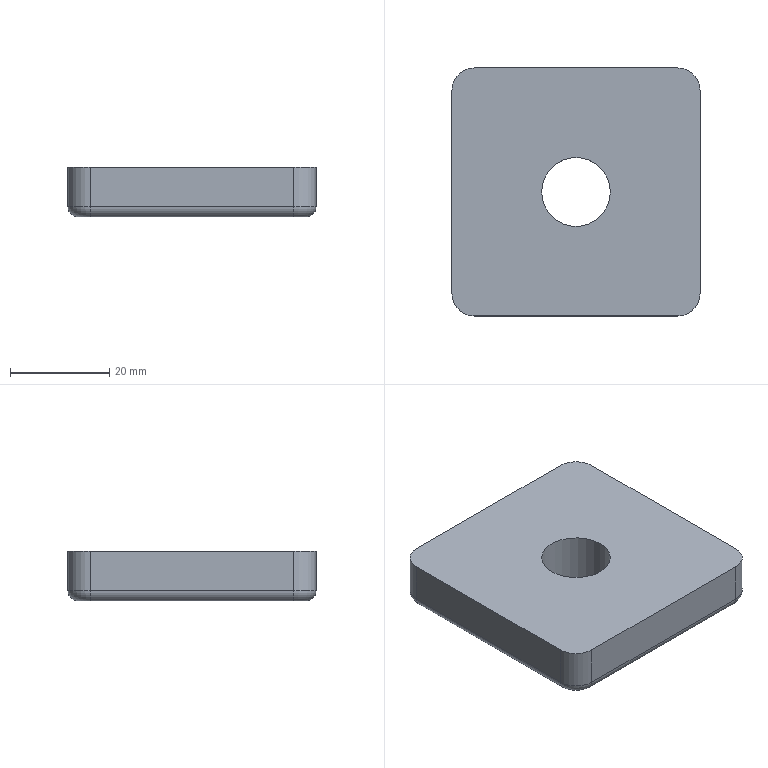Part | STEP file | 14831 | 1 solid | 19 faces | box 50 x 50 x 10 mm | volume 23160 mm3 | cylinder 8 | plane 6 | torus 4 | spline 1 | commonest cylinder face diameters 4 x4 9 x4
STEP:
#1=CARTESIAN_POINT('',(0.,0.,0.));
#2=DIRECTION('',(0.,0.,1.));
#3=DIRECTION('',(1.,0.,0.));
#4=AXIS2_PLACEMENT_3D('',#1,#2,#3);
#5=CARTESIAN_POINT('',(-133.276,-146.636,0.));
#6=VERTEX_POINT('',#5);
#7=CARTESIAN_POINT('',(-133.276,-148.636,2.));
#8=VERTEX_POINT('',#7);
#9=CARTESIAN_POINT('',(-133.276,-146.636,2.));
#10=DIRECTION('',(-1.,0.,0.));
#11=DIRECTION('',(0.,0.,-1.));
#12=AXIS2_PLACEMENT_3D('',#9,#10,#11);
#13=CIRCLE('',#12,2.);
#14=CARTESIAN_POINT('',(-143.526,-146.636,2.));
#15=DIRECTION('',(-1.,0.,0.));
#16=DIRECTION('',(0.,-0.7071,-0.7071));
#17=AXIS2_PLACEMENT_3D('',#14,#15,#16);
#18=CYLINDRICAL_SURFACE('',#17,2.);
#19=CARTESIAN_POINT('',(5.498,-10.25));
#20=DIRECTION('',(1.,0.));
#21=VECTOR('',#20,1.);
#22=LINE('',#19,#21);
#23=(GEOMETRIC_REPRESENTATION_CONTEXT(2)PARAMETRIC_REPRESENTATION_CONTEXT()REPRESENTATION_CONTEXT('',''));
#24=DEFINITIONAL_REPRESENTATION('',(#22),#23);
#25=PCURVE('',#18,#24);
#26=CARTESIAN_POINT('',(-133.276,-144.136,2.));
#27=DIRECTION('',(0.,0.,-1.));
#28=DIRECTION('',(-1.,0.,0.));
#29=AXIS2_PLACEMENT_3D('',#26,#27,#28);
#30=TOROIDAL_SURFACE('',#29,2.5,2.);
#31=CARTESIAN_POINT('',(4.712,1.571));
#32=DIRECTION('',(0.,-1.));
#33=VECTOR('',#32,1.);
#34=LINE('',#31,#33);
#35=(GEOMETRIC_REPRESENTATION_CONTEXT(2)PARAMETRIC_REPRESENTATION_CONTEXT()REPRESENTATION_CONTEXT('',''));
#36=DEFINITIONAL_REPRESENTATION('',(#34),#35);
#37=PCURVE('',#30,#36);
#38=SURFACE_CURVE('',#13,(#25,#37),.PCURVE_S1.);
#39=EDGE_CURVE('',#6,#8,#38,.T.);
#40=ORIENTED_EDGE('',*,*,#39,.T.);
#41=CARTESIAN_POINT('',(-174.276,-148.636,2.));
#42=VERTEX_POINT('',#41);
#43=CARTESIAN_POINT('',(-133.276,-148.636,2.));
#44=DIRECTION('',(-1.,0.,0.));
#45=VECTOR('',#44,1.);
#46=LINE('',#43,#45);
#47=CARTESIAN_POINT('',(7.069,-10.25));
#48=DIRECTION('',(0.,1.));
#49=VECTOR('',#48,1.);
#50=LINE('',#47,#49);
#51=(GEOMETRIC_REPRESENTATION_CONTEXT(2)PARAMETRIC_REPRESENTATION_CONTEXT()REPRESENTATION_CONTEXT('',''));
#52=DEFINITIONAL_REPRESENTATION('',(#50),#51);
#53=PCURVE('',#18,#52);
#54=CARTESIAN_POINT('',(-133.276,-148.636,0.));
#55=DIRECTION('',(0.,-1.,0.));
#56=DIRECTION('',(0.,0.,-1.));
#57=AXIS2_PLACEMENT_3D('',#54,#55,#56);
#58=PLANE('',#57);
#59=CARTESIAN_POINT('',(-2.,0.));
#60=DIRECTION('',(0.,-1.));
#61=VECTOR('',#60,1.);
#62=LINE('',#59,#61);
#63=(GEOMETRIC_REPRESENTATION_CONTEXT(2)PARAMETRIC_REPRESENTATION_CONTEXT()REPRESENTATION_CONTEXT('',''));
#64=DEFINITIONAL_REPRESENTATION('',(#62),#63);
#65=PCURVE('',#58,#64);
#66=SURFACE_CURVE('',#46,(#53,#65),.PCURVE_S1.);
#67=EDGE_CURVE('',#8,#42,#66,.T.);
#68=ORIENTED_EDGE('',*,*,#67,.T.);
#69=CARTESIAN_POINT('',(-174.276,-146.636,0.));
#70=VERTEX_POINT('',#69);
#71=CARTESIAN_POINT('',(-174.276,-146.636,2.));
#72=DIRECTION('',(1.,0.,0.));
#73=DIRECTION('',(0.,-1.,0.));
#74=AXIS2_PLACEMENT_3D('',#71,#72,#73);
#75=CIRCLE('',#74,2.);
#76=CARTESIAN_POINT('',(7.069,30.75));
#77=DIRECTION('',(-1.,0.));
#78=VECTOR('',#77,1.);
#79=LINE('',#76,#78);
#80=(GEOMETRIC_REPRESENTATION_CONTEXT(2)PARAMETRIC_REPRESENTATION_CONTEXT()REPRESENTATION_CONTEXT('',''));
#81=DEFINITIONAL_REPRESENTATION('',(#79),#80);
#82=PCURVE('',#18,#81);
#83=CARTESIAN_POINT('',(-174.276,-144.136,2.));
#84=DIRECTION('',(0.,0.,-1.));
#85=DIRECTION('',(-1.,0.,0.));
#86=AXIS2_PLACEMENT_3D('',#83,#84,#85);
#87=TOROIDAL_SURFACE('',#86,2.5,2.);
#88=CARTESIAN_POINT('',(4.712,0.));
#89=DIRECTION('',(0.,1.));
#90=VECTOR('',#89,1.);
#91=LINE('',#88,#90);
#92=(GEOMETRIC_REPRESENTATION_CONTEXT(2)PARAMETRIC_REPRESENTATION_CONTEXT()REPRESENTATION_CONTEXT('',''));
#93=DEFINITIONAL_REPRESENTATION('',(#91),#92);
#94=PCURVE('',#87,#93);
#95=SURFACE_CURVE('',#75,(#82,#94),.PCURVE_S1.);
#96=EDGE_CURVE('',#42,#70,#95,.T.);
#97=ORIENTED_EDGE('',*,*,#96,.T.);
#98=CARTESIAN_POINT('',(-174.276,-146.636,0.));
#99=DIRECTION('',(1.,0.,0.));
#100=VECTOR('',#99,1.);
#101=LINE('',#98,#100);
#102=CARTESIAN_POINT('',(5.498,30.75));
#103=DIRECTION('',(0.,-1.));
#104=VECTOR('',#103,1.);
#105=LINE('',#102,#104);
#106=(GEOMETRIC_REPRESENTATION_CONTEXT(2)PARAMETRIC_REPRESENTATION_CONTEXT()REPRESENTATION_CONTEXT('',''));
#107=DEFINITIONAL_REPRESENTATION('',(#105),#106);
#108=PCURVE('',#18,#107);
#109=CARTESIAN_POINT('',(-153.776,-123.636,0.));
#110=DIRECTION('',(0.,0.,1.));
#111=DIRECTION('',(1.,0.,0.));
#112=AXIS2_PLACEMENT_3D('',#109,#110,#111);
#113=PLANE('',#112);
#114=CARTESIAN_POINT('',(-20.5,-23.));
#115=DIRECTION('',(1.,0.));
#116=VECTOR('',#115,1.);
#117=LINE('',#114,#116);
#118=(GEOMETRIC_REPRESENTATION_CONTEXT(2)PARAMETRIC_REPRESENTATION_CONTEXT()REPRESENTATION_CONTEXT('',''));
#119=DEFINITIONAL_REPRESENTATION('',(#117),#118);
#120=PCURVE('',#113,#119);
#121=SURFACE_CURVE('',#101,(#108,#120),.PCURVE_S1.);
#122=EDGE_CURVE('',#70,#6,#121,.T.);
#123=ORIENTED_EDGE('',*,*,#122,.T.);
#124=EDGE_LOOP('',(#40,#68,#97,#123));
#125=FACE_BOUND('',#124,.T.);
#126=ADVANCED_FACE('',(#125),#18,.T.);
#127=CARTESIAN_POINT('',(-130.776,-144.136,0.));
#128=VERTEX_POINT('',#127);
#129=CARTESIAN_POINT('',(-128.776,-144.136,2.));
#130=VERTEX_POINT('',#129);
#131=CARTESIAN_POINT('',(-130.776,-144.136,2.));
#132=DIRECTION('',(0.,-1.,0.));
#133=DIRECTION('',(0.,0.,-1.));
#134=AXIS2_PLACEMENT_3D('',#131,#132,#133);
#135=CIRCLE('',#134,2.);
#136=CARTESIAN_POINT('',(3.142,1.571));
#137=DIRECTION('',(0.,-1.));
#138=VECTOR('',#137,1.);
#139=LINE('',#136,#138);
#140=(GEOMETRIC_REPRESENTATION_CONTEXT(2)PARAMETRIC_REPRESENTATION_CONTEXT()REPRESENTATION_CONTEXT('',''));
#141=DEFINITIONAL_REPRESENTATION('',(#139),#140);
#142=PCURVE('',#30,#141);
#143=CARTESIAN_POINT('',(-130.776,-113.386,2.));
#144=DIRECTION('',(0.,-1.,0.));
#145=DIRECTION('',(0.7071,0.,-0.7071));
#146=AXIS2_PLACEMENT_3D('',#143,#144,#145);
#147=CYLINDRICAL_SURFACE('',#146,2.);
#148=CARTESIAN_POINT('',(5.498,30.75));
#149=DIRECTION('',(1.,0.));
#150=VECTOR('',#149,1.);
#151=LINE('',#148,#150);
#152=(GEOMETRIC_REPRESENTATION_CONTEXT(2)PARAMETRIC_REPRESENTATION_CONTEXT()REPRESENTATION_CONTEXT('',''));
#153=DEFINITIONAL_REPRESENTATION('',(#151),#152);
#154=PCURVE('',#147,#153);
#155=SURFACE_CURVE('',#135,(#142,#154),.PCURVE_S1.);
#156=EDGE_CURVE('',#128,#130,#155,.T.);
#157=ORIENTED_EDGE('',*,*,#156,.T.);
#158=CARTESIAN_POINT('',(-133.276,-144.136,2.));
#159=DIRECTION('',(0.,0.,-1.));
#160=DIRECTION('',(0.7071,-0.7071,0.));
#161=AXIS2_PLACEMENT_3D('',#158,#159,#160);
#162=CIRCLE('',#161,4.5);
#163=CARTESIAN_POINT('',(-2.356,0.));
#164=DIRECTION('',(1.,0.));
#165=VECTOR('',#164,1.);
#166=LINE('',#163,#165);
#167=(GEOMETRIC_REPRESENTATION_CONTEXT(2)PARAMETRIC_REPRESENTATION_CONTEXT()REPRESENTATION_CONTEXT('',''));
#168=DEFINITIONAL_REPRESENTATION('',(#166),#167);
#169=PCURVE('',#30,#168);
#170=CARTESIAN_POINT('',(-133.276,-144.136,0.));
#171=DIRECTION('',(0.,0.,1.));
#172=DIRECTION('',(0.,1.,0.));
#173=AXIS2_PLACEMENT_3D('',#170,#171,#172);
#174=CYLINDRICAL_SURFACE('',#173,4.5);
#175=CARTESIAN_POINT('',(10.21,2.));
#176=DIRECTION('',(-1.,0.));
#177=VECTOR('',#176,1.);
#178=LINE('',#175,#177);
#179=(GEOMETRIC_REPRESENTATION_CONTEXT(2)PARAMETRIC_REPRESENTATION_CONTEXT()REPRESENTATION_CONTEXT('',''));
#180=DEFINITIONAL_REPRESENTATION('',(#178),#179);
#181=PCURVE('',#174,#180);
#182=SURFACE_CURVE('',#162,(#169,#181),.PCURVE_S1.);
#183=EDGE_CURVE('',#130,#8,#182,.T.);
#184=ORIENTED_EDGE('',*,*,#183,.T.);
#185=ORIENTED_EDGE('',*,*,#39,.F.);
#186=CARTESIAN_POINT('',(-133.276,-144.136,0.));
#187=DIRECTION('',(0.,0.,1.));
#188=DIRECTION('',(0.7071,-0.7071,0.));
#189=AXIS2_PLACEMENT_3D('',#186,#187,#188);
#190=CIRCLE('',#189,2.5);
#191=CARTESIAN_POINT('',(10.21,1.571));
#192=DIRECTION('',(-1.,0.));
#193=VECTOR('',#192,1.);
#194=LINE('',#191,#193);
#195=(GEOMETRIC_REPRESENTATION_CONTEXT(2)PARAMETRIC_REPRESENTATION_CONTEXT()REPRESENTATION_CONTEXT('',''));
#196=DEFINITIONAL_REPRESENTATION('',(#194),#195);
#197=PCURVE('',#30,#196);
#198=CARTESIAN_POINT('',(20.5,-20.5));
#199=DIRECTION('',(0.7071,-0.7071));
#200=AXIS2_PLACEMENT_2D('',#198,#199);
#201=CIRCLE('',#200,2.5);
#202=(GEOMETRIC_REPRESENTATION_CONTEXT(2)PARAMETRIC_REPRESENTATION_CONTEXT()REPRESENTATION_CONTEXT('',''));
#203=DEFINITIONAL_REPRESENTATION('',(#201),#202);
#204=PCURVE('',#113,#203);
#205=SURFACE_CURVE('',#190,(#197,#204),.PCURVE_S1.);
#206=EDGE_CURVE('',#6,#128,#205,.T.);
#207=ORIENTED_EDGE('',*,*,#206,.T.);
#208=EDGE_LOOP('',(#157,#184,#185,#207));
#209=FACE_BOUND('',#208,.T.);
#210=ADVANCED_FACE('',(#209),#30,.T.);
#211=CARTESIAN_POINT('',(-178.776,-144.136,2.));
#212=VERTEX_POINT('',#211);
#213=CARTESIAN_POINT('',(-176.776,-144.136,0.));
#214=VERTEX_POINT('',#213);
#215=CARTESIAN_POINT('',(-176.776,-144.136,2.));
#216=DIRECTION('',(0.,-1.,0.));
#217=DIRECTION('',(-1.,0.,0.));
#218=AXIS2_PLACEMENT_3D('',#215,#216,#217);
#219=CIRCLE('',#218,2.);
#220=CARTESIAN_POINT('',(6.283,0.));
#221=DIRECTION('',(0.,1.));
#222=VECTOR('',#221,1.);
#223=LINE('',#220,#222);
#224=(GEOMETRIC_REPRESENTATION_CONTEXT(2)PARAMETRIC_REPRESENTATION_CONTEXT()REPRESENTATION_CONTEXT('',''));
#225=DEFINITIONAL_REPRESENTATION('',(#223),#224);
#226=PCURVE('',#87,#225);
#227=CARTESIAN_POINT('',(-176.776,-133.886,2.));
#228=DIRECTION('',(0.,1.,0.));
#229=DIRECTION('',(-0.7071,0.,-0.7071));
#230=AXIS2_PLACEMENT_3D('',#227,#228,#229);
#231=CYLINDRICAL_SURFACE('',#230,2.);
#232=CARTESIAN_POINT('',(7.069,-10.25));
#233=DIRECTION('',(-1.,0.));
#234=VECTOR('',#233,1.);
#235=LINE('',#232,#234);
#236=(GEOMETRIC_REPRESENTATION_CONTEXT(2)PARAMETRIC_REPRESENTATION_CONTEXT()REPRESENTATION_CONTEXT('',''));
#237=DEFINITIONAL_REPRESENTATION('',(#235),#236);
#238=PCURVE('',#231,#237);
#239=SURFACE_CURVE('',#219,(#226,#238),.PCURVE_S1.);
#240=EDGE_CURVE('',#212,#214,#239,.T.);
#241=ORIENTED_EDGE('',*,*,#240,.T.);
#242=CARTESIAN_POINT('',(-174.276,-144.136,0.));
#243=DIRECTION('',(0.,0.,1.));
#244=DIRECTION('',(-0.7071,-0.7071,0.));
#245=AXIS2_PLACEMENT_3D('',#242,#243,#244);
#246=CIRCLE('',#245,2.5);
#247=CARTESIAN_POINT('',(11.781,1.571));
#248=DIRECTION('',(-1.,0.));
#249=VECTOR('',#248,1.);
#250=LINE('',#247,#249);
#251=(GEOMETRIC_REPRESENTATION_CONTEXT(2)PARAMETRIC_REPRESENTATION_CONTEXT()REPRESENTATION_CONTEXT('',''));
#252=DEFINITIONAL_REPRESENTATION('',(#250),#251);
#253=PCURVE('',#87,#252);
#254=CARTESIAN_POINT('',(-20.5,-20.5));
#255=DIRECTION('',(-0.7071,-0.7071));
#256=AXIS2_PLACEMENT_2D('',#254,#255);
#257=CIRCLE('',#256,2.5);
#258=(GEOMETRIC_REPRESENTATION_CONTEXT(2)PARAMETRIC_REPRESENTATION_CONTEXT()REPRESENTATION_CONTEXT('',''));
#259=DEFINITIONAL_REPRESENTATION('',(#257),#258);
#260=PCURVE('',#113,#259);
#261=SURFACE_CURVE('',#246,(#253,#260),.PCURVE_S1.);
#262=EDGE_CURVE('',#214,#70,#261,.T.);
#263=ORIENTED_EDGE('',*,*,#262,.T.);
#264=ORIENTED_EDGE('',*,*,#96,.F.);
#265=CARTESIAN_POINT('',(-174.276,-144.136,2.));
#266=DIRECTION('',(0.,0.,-1.));
#267=DIRECTION('',(-0.7071,-0.7071,0.));
#268=AXIS2_PLACEMENT_3D('',#265,#266,#267);
#269=CIRCLE('',#268,4.5);
#270=CARTESIAN_POINT('',(-0.7854,0.));
#271=DIRECTION('',(1.,0.));
#272=VECTOR('',#271,1.);
#273=LINE('',#270,#272);
#274=(GEOMETRIC_REPRESENTATION_CONTEXT(2)PARAMETRIC_REPRESENTATION_CONTEXT()REPRESENTATION_CONTEXT('',''));
#275=DEFINITIONAL_REPRESENTATION('',(#273),#274);
#276=PCURVE('',#87,#275);
#277=CARTESIAN_POINT('',(-174.276,-144.136,0.));
#278=DIRECTION('',(0.,0.,1.));
#279=DIRECTION('',(1.,0.,0.));
#280=AXIS2_PLACEMENT_3D('',#277,#278,#279);
#281=CYLINDRICAL_SURFACE('',#280,4.5);
#282=CARTESIAN_POINT('',(10.21,2.));
#283=DIRECTION('',(-1.,0.));
#284=VECTOR('',#283,1.);
#285=LINE('',#282,#284);
#286=(GEOMETRIC_REPRESENTATION_CONTEXT(2)PARAMETRIC_REPRESENTATION_CONTEXT()REPRESENTATION_CONTEXT('',''));
#287=DEFINITIONAL_REPRESENTATION('',(#285),#286);
#288=PCURVE('',#281,#287);
#289=SURFACE_CURVE('',#269,(#276,#288),.PCURVE_S1.);
#290=EDGE_CURVE('',#42,#212,#289,.T.);
#291=ORIENTED_EDGE('',*,*,#290,.T.);
#292=EDGE_LOOP('',(#241,#263,#264,#291));
#293=FACE_BOUND('',#292,.T.);
#294=ADVANCED_FACE('',(#293),#87,.T.);
#295=CARTESIAN_POINT('',(-130.776,-103.136,0.));
#296=VERTEX_POINT('',#295);
#297=CARTESIAN_POINT('',(-128.776,-103.136,2.));
#298=VERTEX_POINT('',#297);
#299=CARTESIAN_POINT('',(-130.776,-103.136,2.));
#300=DIRECTION('',(0.,-1.,0.));
#301=DIRECTION('',(0.,0.,-1.));
#302=AXIS2_PLACEMENT_3D('',#299,#300,#301);
#303=CIRCLE('',#302,2.);
#304=CARTESIAN_POINT('',(5.498,-10.25));
#305=DIRECTION('',(1.,0.));
#306=VECTOR('',#305,1.);
#307=LINE('',#304,#306);
#308=(GEOMETRIC_REPRESENTATION_CONTEXT(2)PARAMETRIC_REPRESENTATION_CONTEXT()REPRESENTATION_CONTEXT('',''));
#309=DEFINITIONAL_REPRESENTATION('',(#307),#308);
#310=PCURVE('',#147,#309);
#311=CARTESIAN_POINT('',(-133.276,-103.136,2.));
#312=DIRECTION('',(0.,0.,-1.));
#313=DIRECTION('',(-1.,0.,0.));
#314=AXIS2_PLACEMENT_3D('',#311,#312,#313);
#315=TOROIDAL_SURFACE('',#314,2.5,2.);
#316=CARTESIAN_POINT('',(3.142,1.571));
#317=DIRECTION('',(0.,-1.));
#318=VECTOR('',#317,1.);
#319=LINE('',#316,#318);
#320=(GEOMETRIC_REPRESENTATION_CONTEXT(2)PARAMETRIC_REPRESENTATION_CONTEXT()REPRESENTATION_CONTEXT('',''));
#321=DEFINITIONAL_REPRESENTATION('',(#319),#320);
#322=PCURVE('',#315,#321);
#323=SURFACE_CURVE('',#303,(#310,#322),.PCURVE_S1.);
#324=EDGE_CURVE('',#296,#298,#323,.T.);
#325=ORIENTED_EDGE('',*,*,#324,.T.);
#326=CARTESIAN_POINT('',(-128.776,-103.136,2.));
#327=DIRECTION('',(0.,-1.,0.));
#328=VECTOR('',#327,1.);
#329=LINE('',#326,#328);
#330=CARTESIAN_POINT('',(7.069,-10.25));
#331=DIRECTION('',(0.,1.));
#332=VECTOR('',#331,1.);
#333=LINE('',#330,#332);
#334=(GEOMETRIC_REPRESENTATION_CONTEXT(2)PARAMETRIC_REPRESENTATION_CONTEXT()REPRESENTATION_CONTEXT('',''));
#335=DEFINITIONAL_REPRESENTATION('',(#333),#334);
#336=PCURVE('',#147,#335);
#337=CARTESIAN_POINT('',(-128.776,-103.136,0.));
#338=DIRECTION('',(1.,0.,0.));
#339=DIRECTION('',(0.,0.,-1.));
#340=AXIS2_PLACEMENT_3D('',#337,#338,#339);
#341=PLANE('',#340);
#342=CARTESIAN_POINT('',(-2.,0.));
#343=DIRECTION('',(0.,-1.));
#344=VECTOR('',#343,1.);
#345=LINE('',#342,#344);
#346=(GEOMETRIC_REPRESENTATION_CONTEXT(2)PARAMETRIC_REPRESENTATION_CONTEXT()REPRESENTATION_CONTEXT('',''));
#347=DEFINITIONAL_REPRESENTATION('',(#345),#346);
#348=PCURVE('',#341,#347);
#349=SURFACE_CURVE('',#329,(#336,#348),.PCURVE_S1.);
#350=EDGE_CURVE('',#298,#130,#349,.T.);
#351=ORIENTED_EDGE('',*,*,#350,.T.);
#352=ORIENTED_EDGE('',*,*,#156,.F.);
#353=CARTESIAN_POINT('',(-130.776,-144.136,0.));
#354=DIRECTION('',(0.,1.,0.));
#355=VECTOR('',#354,1.);
#356=LINE('',#353,#355);
#357=CARTESIAN_POINT('',(5.498,30.75));
#358=DIRECTION('',(0.,-1.));
#359=VECTOR('',#358,1.);
#360=LINE('',#357,#359);
#361=(GEOMETRIC_REPRESENTATION_CONTEXT(2)PARAMETRIC_REPRESENTATION_CONTEXT()REPRESENTATION_CONTEXT('',''));
#362=DEFINITIONAL_REPRESENTATION('',(#360),#361);
#363=PCURVE('',#147,#362);
#364=CARTESIAN_POINT('',(23.,-20.5));
#365=DIRECTION('',(0.,1.));
#366=VECTOR('',#365,1.);
#367=LINE('',#364,#366);
#368=(GEOMETRIC_REPRESENTATION_CONTEXT(2)PARAMETRIC_REPRESENTATION_CONTEXT()REPRESENTATION_CONTEXT('',''));
#369=DEFINITIONAL_REPRESENTATION('',(#367),#368);
#370=PCURVE('',#113,#369);
#371=SURFACE_CURVE('',#356,(#363,#370),.PCURVE_S1.);
#372=EDGE_CURVE('',#128,#296,#371,.T.);
#373=ORIENTED_EDGE('',*,*,#372,.T.);
#374=EDGE_LOOP('',(#325,#351,#352,#373));
#375=FACE_BOUND('',#374,.T.);
#376=ADVANCED_FACE('',(#375),#147,.T.);
#377=CARTESIAN_POINT('',(-178.776,-103.136,2.));
#378=VERTEX_POINT('',#377);
#379=CARTESIAN_POINT('',(-176.776,-103.136,0.));
#380=VERTEX_POINT('',#379);
#381=CARTESIAN_POINT('',(-176.776,-103.136,2.));
#382=DIRECTION('',(0.,-1.,0.));
#383=DIRECTION('',(-1.,0.,0.));
#384=AXIS2_PLACEMENT_3D('',#381,#382,#383);
#385=CIRCLE('',#384,2.);
#386=CARTESIAN_POINT('',(7.069,30.75));
#387=DIRECTION('',(-1.,0.));
#388=VECTOR('',#387,1.);
#389=LINE('',#386,#388);
#390=(GEOMETRIC_REPRESENTATION_CONTEXT(2)PARAMETRIC_REPRESENTATION_CONTEXT()REPRESENTATION_CONTEXT('',''));
#391=DEFINITIONAL_REPRESENTATION('',(#389),#390);
#392=PCURVE('',#231,#391);
#393=CARTESIAN_POINT('',(-174.276,-103.136,2.));
#394=DIRECTION('',(0.,0.,-1.));
#395=DIRECTION('',(-1.,0.,0.));
#396=AXIS2_PLACEMENT_3D('',#393,#394,#395);
#397=TOROIDAL_SURFACE('',#396,2.5,2.);
#398=CARTESIAN_POINT('',(0.,0.));
#399=DIRECTION('',(0.,1.));
#400=VECTOR('',#399,1.);
#401=LINE('',#398,#400);
#402=(GEOMETRIC_REPRESENTATION_CONTEXT(2)PARAMETRIC_REPRESENTATION_CONTEXT()REPRESENTATION_CONTEXT('',''));
#403=DEFINITIONAL_REPRESENTATION('',(#401),#402);
#404=PCURVE('',#397,#403);
#405=SURFACE_CURVE('',#385,(#392,#404),.PCURVE_S1.);
#406=EDGE_CURVE('',#378,#380,#405,.T.);
#407=ORIENTED_EDGE('',*,*,#406,.T.);
#408=CARTESIAN_POINT('',(-176.776,-103.136,0.));
#409=DIRECTION('',(0.,-1.,0.));
#410=VECTOR('',#409,1.);
#411=LINE('',#408,#410);
#412=CARTESIAN_POINT('',(5.498,30.75));
#413=DIRECTION('',(0.,-1.));
#414=VECTOR('',#413,1.);
#415=LINE('',#412,#414);
#416=(GEOMETRIC_REPRESENTATION_CONTEXT(2)PARAMETRIC_REPRESENTATION_CONTEXT()REPRESENTATION_CONTEXT('',''));
#417=DEFINITIONAL_REPRESENTATION('',(#415),#416);
#418=PCURVE('',#231,#417);
#419=CARTESIAN_POINT('',(-23.,20.5));
#420=DIRECTION('',(0.,-1.));
#421=VECTOR('',#420,1.);
#422=LINE('',#419,#421);
#423=(GEOMETRIC_REPRESENTATION_CONTEXT(2)PARAMETRIC_REPRESENTATION_CONTEXT()REPRESENTATION_CONTEXT('',''));
#424=DEFINITIONAL_REPRESENTATION('',(#422),#423);
#425=PCURVE('',#113,#424);
#426=SURFACE_CURVE('',#411,(#418,#425),.PCURVE_S1.);
#427=EDGE_CURVE('',#380,#214,#426,.T.);
#428=ORIENTED_EDGE('',*,*,#427,.T.);
#429=ORIENTED_EDGE('',*,*,#240,.F.);
#430=CARTESIAN_POINT('',(-178.776,-144.136,2.));
#431=DIRECTION('',(0.,1.,0.));
#432=VECTOR('',#431,1.);
#433=LINE('',#430,#432);
#434=CARTESIAN_POINT('',(7.069,-10.25));
#435=DIRECTION('',(0.,1.));
#436=VECTOR('',#435,1.);
#437=LINE('',#434,#436);
#438=(GEOMETRIC_REPRESENTATION_CONTEXT(2)PARAMETRIC_REPRESENTATION_CONTEXT()REPRESENTATION_CONTEXT('',''));
#439=DEFINITIONAL_REPRESENTATION('',(#437),#438);
#440=PCURVE('',#231,#439);
#441=CARTESIAN_POINT('',(-178.776,-144.136,0.));
#442=DIRECTION('',(-1.,0.,0.));
#443=DIRECTION('',(0.,0.,1.));
#444=AXIS2_PLACEMENT_3D('',#441,#442,#443);
#445=PLANE('',#444);
#446=CARTESIAN_POINT('',(2.,0.));
#447=DIRECTION('',(0.,1.));
#448=VECTOR('',#447,1.);
#449=LINE('',#446,#448);
#450=(GEOMETRIC_REPRESENTATION_CONTEXT(2)PARAMETRIC_REPRESENTATION_CONTEXT()REPRESENTATION_CONTEXT('',''));
#451=DEFINITIONAL_REPRESENTATION('',(#449),#450);
#452=PCURVE('',#445,#451);
#453=SURFACE_CURVE('',#433,(#440,#452),.PCURVE_S1.);
#454=EDGE_CURVE('',#212,#378,#453,.T.);
#455=ORIENTED_EDGE('',*,*,#454,.T.);
#456=EDGE_LOOP('',(#407,#428,#429,#455));
#457=FACE_BOUND('',#456,.T.);
#458=ADVANCED_FACE('',(#457),#231,.T.);
#459=CARTESIAN_POINT('',(-133.276,-100.636,0.));
#460=VERTEX_POINT('',#459);
#461=CARTESIAN_POINT('',(-133.276,-98.636,2.));
#462=VERTEX_POINT('',#461);
#463=CARTESIAN_POINT('',(-133.276,-100.636,2.));
#464=DIRECTION('',(1.,0.,0.));
#465=DIRECTION('',(0.,0.,-1.));
#466=AXIS2_PLACEMENT_3D('',#463,#464,#465);
#467=CIRCLE('',#466,2.);
#468=CARTESIAN_POINT('',(1.571,1.571));
#469=DIRECTION('',(0.,-1.));
#470=VECTOR('',#469,1.);
#471=LINE('',#468,#470);
#472=(GEOMETRIC_REPRESENTATION_CONTEXT(2)PARAMETRIC_REPRESENTATION_CONTEXT()REPRESENTATION_CONTEXT('',''));
#473=DEFINITIONAL_REPRESENTATION('',(#471),#472);
#474=PCURVE('',#315,#473);
#475=CARTESIAN_POINT('',(-164.026,-100.636,2.));
#476=DIRECTION('',(1.,0.,0.));
#477=DIRECTION('',(0.,0.7071,-0.7071));
#478=AXIS2_PLACEMENT_3D('',#475,#476,#477);
#479=CYLINDRICAL_SURFACE('',#478,2.);
#480=CARTESIAN_POINT('',(5.498,30.75));
#481=DIRECTION('',(1.,0.));
#482=VECTOR('',#481,1.);
#483=LINE('',#480,#482);
#484=(GEOMETRIC_REPRESENTATION_CONTEXT(2)PARAMETRIC_REPRESENTATION_CONTEXT()REPRESENTATION_CONTEXT('',''));
#485=DEFINITIONAL_REPRESENTATION('',(#483),#484);
#486=PCURVE('',#479,#485);
#487=SURFACE_CURVE('',#467,(#474,#486),.PCURVE_S1.);
#488=EDGE_CURVE('',#460,#462,#487,.T.);
#489=ORIENTED_EDGE('',*,*,#488,.T.);
#490=CARTESIAN_POINT('',(-133.276,-103.136,2.));
#491=DIRECTION('',(0.,0.,-1.));
#492=DIRECTION('',(0.7071,0.7071,0.));
#493=AXIS2_PLACEMENT_3D('',#490,#491,#492);
#494=CIRCLE('',#493,4.5);
#495=CARTESIAN_POINT('',(-3.927,0.));
#496=DIRECTION('',(1.,0.));
#497=VECTOR('',#496,1.);
#498=LINE('',#495,#497);
#499=(GEOMETRIC_REPRESENTATION_CONTEXT(2)PARAMETRIC_REPRESENTATION_CONTEXT()REPRESENTATION_CONTEXT('',''));
#500=DEFINITIONAL_REPRESENTATION('',(#498),#499);
#501=PCURVE('',#315,#500);
#502=CARTESIAN_POINT('',(-133.276,-103.136,0.));
#503=DIRECTION('',(0.,0.,1.));
#504=DIRECTION('',(-1.,0.,0.));
#505=AXIS2_PLACEMENT_3D('',#502,#503,#504);
#506=CYLINDRICAL_SURFACE('',#505,4.5);
#507=CARTESIAN_POINT('',(10.21,2.));
#508=DIRECTION('',(-1.,0.));
#509=VECTOR('',#508,1.);
#510=LINE('',#507,#509);
#511=(GEOMETRIC_REPRESENTATION_CONTEXT(2)PARAMETRIC_REPRESENTATION_CONTEXT()REPRESENTATION_CONTEXT('',''));
#512=DEFINITIONAL_REPRESENTATION('',(#510),#511);
#513=PCURVE('',#506,#512);
#514=SURFACE_CURVE('',#494,(#501,#513),.PCURVE_S1.);
#515=EDGE_CURVE('',#462,#298,#514,.T.);
#516=ORIENTED_EDGE('',*,*,#515,.T.);
#517=ORIENTED_EDGE('',*,*,#324,.F.);
#518=CARTESIAN_POINT('',(-133.276,-103.136,0.));
#519=DIRECTION('',(0.,0.,1.));
#520=DIRECTION('',(0.7071,0.7071,0.));
#521=AXIS2_PLACEMENT_3D('',#518,#519,#520);
#522=CIRCLE('',#521,2.5);
#523=CARTESIAN_POINT('',(8.639,1.571));
#524=DIRECTION('',(-1.,0.));
#525=VECTOR('',#524,1.);
#526=LINE('',#523,#525);
#527=(GEOMETRIC_REPRESENTATION_CONTEXT(2)PARAMETRIC_REPRESENTATION_CONTEXT()REPRESENTATION_CONTEXT('',''));
#528=DEFINITIONAL_REPRESENTATION('',(#526),#527);
#529=PCURVE('',#315,#528);
#530=CARTESIAN_POINT('',(20.5,20.5));
#531=DIRECTION('',(0.7071,0.7071));
#532=AXIS2_PLACEMENT_2D('',#530,#531);
#533=CIRCLE('',#532,2.5);
#534=(GEOMETRIC_REPRESENTATION_CONTEXT(2)PARAMETRIC_REPRESENTATION_CONTEXT()REPRESENTATION_CONTEXT('',''));
#535=DEFINITIONAL_REPRESENTATION('',(#533),#534);
#536=PCURVE('',#113,#535);
#537=SURFACE_CURVE('',#522,(#529,#536),.PCURVE_S1.);
#538=EDGE_CURVE('',#296,#460,#537,.T.);
#539=ORIENTED_EDGE('',*,*,#538,.T.);
#540=EDGE_LOOP('',(#489,#516,#517,#539));
#541=FACE_BOUND('',#540,.T.);
#542=ADVANCED_FACE('',(#541),#315,.T.);
#543=CARTESIAN_POINT('',(-174.276,-98.636,2.));
#544=VERTEX_POINT('',#543);
#545=CARTESIAN_POINT('',(-174.276,-100.636,0.));
#546=VERTEX_POINT('',#545);
#547=CARTESIAN_POINT('',(-174.276,-100.636,2.));
#548=DIRECTION('',(-1.,0.,0.));
#549=DIRECTION('',(0.,1.,0.));
#550=AXIS2_PLACEMENT_3D('',#547,#548,#549);
#551=CIRCLE('',#550,2.);
#552=CARTESIAN_POINT('',(1.571,0.));
#553=DIRECTION('',(0.,1.));
#554=VECTOR('',#553,1.);
#555=LINE('',#552,#554);
#556=(GEOMETRIC_REPRESENTATION_CONTEXT(2)PARAMETRIC_REPRESENTATION_CONTEXT()REPRESENTATION_CONTEXT('',''));
#557=DEFINITIONAL_REPRESENTATION('',(#555),#556);
#558=PCURVE('',#397,#557);
#559=CARTESIAN_POINT('',(7.069,-10.25));
#560=DIRECTION('',(-1.,0.));
#561=VECTOR('',#560,1.);
#562=LINE('',#559,#561);
#563=(GEOMETRIC_REPRESENTATION_CONTEXT(2)PARAMETRIC_REPRESENTATION_CONTEXT()REPRESENTATION_CONTEXT('',''));
#564=DEFINITIONAL_REPRESENTATION('',(#562),#563);
#565=PCURVE('',#479,#564);
#566=SURFACE_CURVE('',#551,(#558,#565),.PCURVE_S1.);
#567=EDGE_CURVE('',#544,#546,#566,.T.);
#568=ORIENTED_EDGE('',*,*,#567,.T.);
#569=CARTESIAN_POINT('',(-174.276,-103.136,0.));
#570=DIRECTION('',(0.,0.,1.));
#571=DIRECTION('',(-0.7071,0.7071,0.));
#572=AXIS2_PLACEMENT_3D('',#569,#570,#571);
#573=CIRCLE('',#572,2.5);
#574=CARTESIAN_POINT('',(7.069,1.571));
#575=DIRECTION('',(-1.,0.));
#576=VECTOR('',#575,1.);
#577=LINE('',#574,#576);
#578=(GEOMETRIC_REPRESENTATION_CONTEXT(2)PARAMETRIC_REPRESENTATION_CONTEXT()REPRESENTATION_CONTEXT('',''));
#579=DEFINITIONAL_REPRESENTATION('',(#577),#578);
#580=PCURVE('',#397,#579);
#581=CARTESIAN_POINT('',(-20.5,20.5));
#582=DIRECTION('',(-0.7071,0.7071));
#583=AXIS2_PLACEMENT_2D('',#581,#582);
#584=CIRCLE('',#583,2.5);
#585=(GEOMETRIC_REPRESENTATION_CONTEXT(2)PARAMETRIC_REPRESENTATION_CONTEXT()REPRESENTATION_CONTEXT('',''));
#586=DEFINITIONAL_REPRESENTATION('',(#584),#585);
#587=PCURVE('',#113,#586);
#588=SURFACE_CURVE('',#573,(#580,#587),.PCURVE_S1.);
#589=EDGE_CURVE('',#546,#380,#588,.T.);
#590=ORIENTED_EDGE('',*,*,#589,.T.);
#591=ORIENTED_EDGE('',*,*,#406,.F.);
#592=CARTESIAN_POINT('',(-174.276,-103.136,2.));
#593=DIRECTION('',(0.,0.,-1.));
#594=DIRECTION('',(-0.7071,0.7071,0.));
#595=AXIS2_PLACEMENT_3D('',#592,#593,#594);
#596=CIRCLE('',#595,4.5);
#597=CARTESIAN_POINT('',(-5.498,0.));
#598=DIRECTION('',(1.,0.));
#599=VECTOR('',#598,1.);
#600=LINE('',#597,#599);
#601=(GEOMETRIC_REPRESENTATION_CONTEXT(2)PARAMETRIC_REPRESENTATION_CONTEXT()REPRESENTATION_CONTEXT('',''));
#602=DEFINITIONAL_REPRESENTATION('',(#600),#601);
#603=PCURVE('',#397,#602);
#604=CARTESIAN_POINT('',(-174.276,-103.136,0.));
#605=DIRECTION('',(0.,0.,1.));
#606=DIRECTION('',(0.,-1.,0.));
#607=AXIS2_PLACEMENT_3D('',#604,#605,#606);
#608=CYLINDRICAL_SURFACE('',#607,4.5);
#609=CARTESIAN_POINT('',(10.21,2.));
#610=DIRECTION('',(-1.,0.));
#611=VECTOR('',#610,1.);
#612=LINE('',#609,#611);
#613=(GEOMETRIC_REPRESENTATION_CONTEXT(2)PARAMETRIC_REPRESENTATION_CONTEXT()REPRESENTATION_CONTEXT('',''));
#614=DEFINITIONAL_REPRESENTATION('',(#612),#613);
#615=PCURVE('',#608,#614);
#616=SURFACE_CURVE('',#596,(#603,#615),.PCURVE_S1.);
#617=EDGE_CURVE('',#378,#544,#616,.T.);
#618=ORIENTED_EDGE('',*,*,#617,.T.);
#619=EDGE_LOOP('',(#568,#590,#591,#618));
#620=FACE_BOUND('',#619,.T.);
#621=ADVANCED_FACE('',(#620),#397,.T.);
#622=ORIENTED_EDGE('',*,*,#488,.F.);
#623=CARTESIAN_POINT('',(-133.276,-100.636,0.));
#624=DIRECTION('',(-1.,0.,0.));
#625=VECTOR('',#624,1.);
#626=LINE('',#623,#625);
#627=CARTESIAN_POINT('',(5.498,30.75));
#628=DIRECTION('',(0.,-1.));
#629=VECTOR('',#628,1.);
#630=LINE('',#627,#629);
#631=(GEOMETRIC_REPRESENTATION_CONTEXT(2)PARAMETRIC_REPRESENTATION_CONTEXT()REPRESENTATION_CONTEXT('',''));
#632=DEFINITIONAL_REPRESENTATION('',(#630),#631);
#633=PCURVE('',#479,#632);
#634=CARTESIAN_POINT('',(20.5,23.));
#635=DIRECTION('',(-1.,0.));
#636=VECTOR('',#635,1.);
#637=LINE('',#634,#636);
#638=(GEOMETRIC_REPRESENTATION_CONTEXT(2)PARAMETRIC_REPRESENTATION_CONTEXT()REPRESENTATION_CONTEXT('',''));
#639=DEFINITIONAL_REPRESENTATION('',(#637),#638);
#640=PCURVE('',#113,#639);
#641=SURFACE_CURVE('',#626,(#633,#640),.PCURVE_S1.);
#642=EDGE_CURVE('',#460,#546,#641,.T.);
#643=ORIENTED_EDGE('',*,*,#642,.T.);
#644=ORIENTED_EDGE('',*,*,#567,.F.);
#645=CARTESIAN_POINT('',(-174.276,-98.636,2.));
#646=DIRECTION('',(1.,0.,0.));
#647=VECTOR('',#646,1.);
#648=LINE('',#645,#647);
#649=CARTESIAN_POINT('',(7.069,-10.25));
#650=DIRECTION('',(0.,1.));
#651=VECTOR('',#650,1.);
#652=LINE('',#649,#651);
#653=(GEOMETRIC_REPRESENTATION_CONTEXT(2)PARAMETRIC_REPRESENTATION_CONTEXT()REPRESENTATION_CONTEXT('',''));
#654=DEFINITIONAL_REPRESENTATION('',(#652),#653);
#655=PCURVE('',#479,#654);
#656=CARTESIAN_POINT('',(-174.276,-98.636,0.));
#657=DIRECTION('',(0.,1.,0.));
#658=DIRECTION('',(0.,0.,1.));
#659=AXIS2_PLACEMENT_3D('',#656,#657,#658);
#660=PLANE('',#659);
#661=CARTESIAN_POINT('',(2.,0.));
#662=DIRECTION('',(0.,1.));
#663=VECTOR('',#662,1.);
#664=LINE('',#661,#663);
#665=(GEOMETRIC_REPRESENTATION_CONTEXT(2)PARAMETRIC_REPRESENTATION_CONTEXT()REPRESENTATION_CONTEXT('',''));
#666=DEFINITIONAL_REPRESENTATION('',(#664),#665);
#667=PCURVE('',#660,#666);
#668=SURFACE_CURVE('',#648,(#655,#667),.PCURVE_S1.);
#669=EDGE_CURVE('',#544,#462,#668,.T.);
#670=ORIENTED_EDGE('',*,*,#669,.T.);
#671=EDGE_LOOP('',(#622,#643,#644,#670));
#672=FACE_BOUND('',#671,.T.);
#673=ADVANCED_FACE('',(#672),#479,.T.);
#674=ORIENTED_EDGE('',*,*,#617,.F.);
#675=CARTESIAN_POINT('',(-178.776,-103.136,10.));
#676=VERTEX_POINT('',#675);
#677=CARTESIAN_POINT('',(-178.776,-103.136,2.));
#678=DIRECTION('',(0.,0.,1.));
#679=VECTOR('',#678,1.);
#680=LINE('',#677,#679);
#681=CARTESIAN_POINT('',(4.712,2.));
#682=DIRECTION('',(0.,1.));
#683=VECTOR('',#682,1.);
#684=LINE('',#681,#683);
#685=(GEOMETRIC_REPRESENTATION_CONTEXT(2)PARAMETRIC_REPRESENTATION_CONTEXT()REPRESENTATION_CONTEXT('',''));
#686=DEFINITIONAL_REPRESENTATION('',(#684),#685);
#687=PCURVE('',#608,#686);
#688=CARTESIAN_POINT('',(2.,41.));
#689=DIRECTION('',(1.,0.));
#690=VECTOR('',#689,1.);
#691=LINE('',#688,#690);
#692=(GEOMETRIC_REPRESENTATION_CONTEXT(2)PARAMETRIC_REPRESENTATION_CONTEXT()REPRESENTATION_CONTEXT('',''));
#693=DEFINITIONAL_REPRESENTATION('',(#691),#692);
#694=PCURVE('',#445,#693);
#695=SURFACE_CURVE('',#680,(#687,#694),.PCURVE_S1.);
#696=EDGE_CURVE('',#378,#676,#695,.T.);
#697=ORIENTED_EDGE('',*,*,#696,.T.);
#698=CARTESIAN_POINT('',(-174.276,-98.636,10.));
#699=VERTEX_POINT('',#698);
#700=CARTESIAN_POINT('',(-174.276,-103.136,10.));
#701=DIRECTION('',(0.,0.,-1.));
#702=DIRECTION('',(0.,-1.,0.));
#703=AXIS2_PLACEMENT_3D('',#700,#701,#702);
#704=CIRCLE('',#703,4.5);
#705=CARTESIAN_POINT('',(6.283,10.));
#706=DIRECTION('',(-1.,0.));
#707=VECTOR('',#706,1.);
#708=LINE('',#705,#707);
#709=(GEOMETRIC_REPRESENTATION_CONTEXT(2)PARAMETRIC_REPRESENTATION_CONTEXT()REPRESENTATION_CONTEXT('',''));
#710=DEFINITIONAL_REPRESENTATION('',(#708),#709);
#711=PCURVE('',#608,#710);
#712=CARTESIAN_POINT('',(-153.776,-123.636,10.));
#713=DIRECTION('',(0.,0.,1.));
#714=DIRECTION('',(1.,0.,0.));
#715=AXIS2_PLACEMENT_3D('',#712,#713,#714);
#716=PLANE('',#715);
#717=CARTESIAN_POINT('',(-20.5,16.));
#718=CARTESIAN_POINT('',(-28.294,16.));
#719=CARTESIAN_POINT('',(-24.397,22.75));
#720=CARTESIAN_POINT('',(-20.5,29.5));
#721=CARTESIAN_POINT('',(-16.603,22.75));
#722=CARTESIAN_POINT('',(-12.706,16.));
#723=CARTESIAN_POINT('',(-20.5,16.));
#724=(BOUNDED_CURVE()B_SPLINE_CURVE(2,(#717,#718,#719,#720,#721,#722,#723),.UNSPECIFIED.,.T.,.F.)B_SPLINE_CURVE_WITH_KNOTS((1,2,2,2,2,1),(-2.094,0.,2.094,4.189,6.283,8.378),.UNSPECIFIED.)CURVE()GEOMETRIC_REPRESENTATION_ITEM()RATIONAL_B_SPLINE_CURVE((1.,0.5,1.,0.5,1.,0.5,1.))REPRESENTATION_ITEM(''));
#725=(GEOMETRIC_REPRESENTATION_CONTEXT(2)PARAMETRIC_REPRESENTATION_CONTEXT()REPRESENTATION_CONTEXT('',''));
#726=DEFINITIONAL_REPRESENTATION('',(#724),#725);
#727=PCURVE('',#716,#726);
#728=SURFACE_CURVE('',#704,(#711,#727),.PCURVE_S1.);
#729=EDGE_CURVE('',#676,#699,#728,.T.);
#730=ORIENTED_EDGE('',*,*,#729,.T.);
#731=CARTESIAN_POINT('',(-174.276,-98.636,2.));
#732=DIRECTION('',(0.,0.,1.));
#733=VECTOR('',#732,1.);
#734=LINE('',#731,#733);
#735=CARTESIAN_POINT('',(3.142,2.));
#736=DIRECTION('',(0.,1.));
#737=VECTOR('',#736,1.);
#738=LINE('',#735,#737);
#739=(GEOMETRIC_REPRESENTATION_CONTEXT(2)PARAMETRIC_REPRESENTATION_CONTEXT()REPRESENTATION_CONTEXT('',''));
#740=DEFINITIONAL_REPRESENTATION('',(#738),#739);
#741=PCURVE('',#608,#740);
#742=CARTESIAN_POINT('',(2.,0.));
#743=DIRECTION('',(1.,0.));
#744=VECTOR('',#743,1.);
#745=LINE('',#742,#744);
#746=(GEOMETRIC_REPRESENTATION_CONTEXT(2)PARAMETRIC_REPRESENTATION_CONTEXT()REPRESENTATION_CONTEXT('',''));
#747=DEFINITIONAL_REPRESENTATION('',(#745),#746);
#748=PCURVE('',#660,#747);
#749=SURFACE_CURVE('',#734,(#741,#748),.PCURVE_S1.);
#750=EDGE_CURVE('',#544,#699,#749,.T.);
#751=ORIENTED_EDGE('',*,*,#750,.F.);
#752=EDGE_LOOP('',(#674,#697,#730,#751));
#753=FACE_BOUND('',#752,.T.);
#754=ADVANCED_FACE('',(#753),#608,.T.);
#755=ORIENTED_EDGE('',*,*,#454,.F.);
#756=CARTESIAN_POINT('',(-178.776,-144.136,10.));
#757=VERTEX_POINT('',#756);
#758=CARTESIAN_POINT('',(-178.776,-144.136,2.));
#759=DIRECTION('',(0.,0.,1.));
#760=VECTOR('',#759,1.);
#761=LINE('',#758,#760);
#762=CARTESIAN_POINT('',(2.,0.));
#763=DIRECTION('',(1.,0.));
#764=VECTOR('',#763,1.);
#765=LINE('',#762,#764);
#766=(GEOMETRIC_REPRESENTATION_CONTEXT(2)PARAMETRIC_REPRESENTATION_CONTEXT()REPRESENTATION_CONTEXT('',''));
#767=DEFINITIONAL_REPRESENTATION('',(#765),#766);
#768=PCURVE('',#445,#767);
#769=CARTESIAN_POINT('',(3.142,2.));
#770=DIRECTION('',(0.,1.));
#771=VECTOR('',#770,1.);
#772=LINE('',#769,#771);
#773=(GEOMETRIC_REPRESENTATION_CONTEXT(2)PARAMETRIC_REPRESENTATION_CONTEXT()REPRESENTATION_CONTEXT('',''));
#774=DEFINITIONAL_REPRESENTATION('',(#772),#773);
#775=PCURVE('',#281,#774);
#776=SURFACE_CURVE('',#761,(#768,#775),.PCURVE_S1.);
#777=EDGE_CURVE('',#212,#757,#776,.T.);
#778=ORIENTED_EDGE('',*,*,#777,.T.);
#779=CARTESIAN_POINT('',(-178.776,-144.136,10.));
#780=DIRECTION('',(0.,1.,0.));
#781=VECTOR('',#780,1.);
#782=LINE('',#779,#781);
#783=CARTESIAN_POINT('',(10.,0.));
#784=DIRECTION('',(0.,1.));
#785=VECTOR('',#784,1.);
#786=LINE('',#783,#785);
#787=(GEOMETRIC_REPRESENTATION_CONTEXT(2)PARAMETRIC_REPRESENTATION_CONTEXT()REPRESENTATION_CONTEXT('',''));
#788=DEFINITIONAL_REPRESENTATION('',(#786),#787);
#789=PCURVE('',#445,#788);
#790=CARTESIAN_POINT('',(-25.,-20.5));
#791=DIRECTION('',(0.,1.));
#792=VECTOR('',#791,1.);
#793=LINE('',#790,#792);
#794=(GEOMETRIC_REPRESENTATION_CONTEXT(2)PARAMETRIC_REPRESENTATION_CONTEXT()REPRESENTATION_CONTEXT('',''));
#795=DEFINITIONAL_REPRESENTATION('',(#793),#794);
#796=PCURVE('',#716,#795);
#797=SURFACE_CURVE('',#782,(#789,#796),.PCURVE_S1.);
#798=EDGE_CURVE('',#757,#676,#797,.T.);
#799=ORIENTED_EDGE('',*,*,#798,.T.);
#800=ORIENTED_EDGE('',*,*,#696,.F.);
#801=EDGE_LOOP('',(#755,#778,#799,#800));
#802=FACE_BOUND('',#801,.T.);
#803=ADVANCED_FACE('',(#802),#445,.T.);
#804=ORIENTED_EDGE('',*,*,#290,.F.);
#805=CARTESIAN_POINT('',(-174.276,-148.636,10.));
#806=VERTEX_POINT('',#805);
#807=CARTESIAN_POINT('',(-174.276,-148.636,2.));
#808=DIRECTION('',(0.,0.,1.));
#809=VECTOR('',#808,1.);
#810=LINE('',#807,#809);
#811=CARTESIAN_POINT('',(4.712,2.));
#812=DIRECTION('',(0.,1.));
#813=VECTOR('',#812,1.);
#814=LINE('',#811,#813);
#815=(GEOMETRIC_REPRESENTATION_CONTEXT(2)PARAMETRIC_REPRESENTATION_CONTEXT()REPRESENTATION_CONTEXT('',''));
#816=DEFINITIONAL_REPRESENTATION('',(#814),#815);
#817=PCURVE('',#281,#816);
#818=CARTESIAN_POINT('',(-2.,-41.));
#819=DIRECTION('',(-1.,0.));
#820=VECTOR('',#819,1.);
#821=LINE('',#818,#820);
#822=(GEOMETRIC_REPRESENTATION_CONTEXT(2)PARAMETRIC_REPRESENTATION_CONTEXT()REPRESENTATION_CONTEXT('',''));
#823=DEFINITIONAL_REPRESENTATION('',(#821),#822);
#824=PCURVE('',#58,#823);
#825=SURFACE_CURVE('',#810,(#817,#824),.PCURVE_S1.);
#826=EDGE_CURVE('',#42,#806,#825,.T.);
#827=ORIENTED_EDGE('',*,*,#826,.T.);
#828=CARTESIAN_POINT('',(-174.276,-144.136,10.));
#829=DIRECTION('',(0.,0.,-1.));
#830=DIRECTION('',(1.,0.,0.));
#831=AXIS2_PLACEMENT_3D('',#828,#829,#830);
#832=CIRCLE('',#831,4.5);
#833=CARTESIAN_POINT('',(6.283,10.));
#834=DIRECTION('',(-1.,0.));
#835=VECTOR('',#834,1.);
#836=LINE('',#833,#835);
#837=(GEOMETRIC_REPRESENTATION_CONTEXT(2)PARAMETRIC_REPRESENTATION_CONTEXT()REPRESENTATION_CONTEXT('',''));
#838=DEFINITIONAL_REPRESENTATION('',(#836),#837);
#839=PCURVE('',#281,#838);
#840=CARTESIAN_POINT('',(-16.,-20.5));
#841=CARTESIAN_POINT('',(-16.,-28.294));
#842=CARTESIAN_POINT('',(-22.75,-24.397));
#843=CARTESIAN_POINT('',(-29.5,-20.5));
#844=CARTESIAN_POINT('',(-22.75,-16.603));
#845=CARTESIAN_POINT('',(-16.,-12.706));
#846=CARTESIAN_POINT('',(-16.,-20.5));
#847=(BOUNDED_CURVE()B_SPLINE_CURVE(2,(#840,#841,#842,#843,#844,#845,#846),.UNSPECIFIED.,.T.,.F.)B_SPLINE_CURVE_WITH_KNOTS((1,2,2,2,2,1),(-2.094,0.,2.094,4.189,6.283,8.378),.UNSPECIFIED.)CURVE()GEOMETRIC_REPRESENTATION_ITEM()RATIONAL_B_SPLINE_CURVE((1.,0.5,1.,0.5,1.,0.5,1.))REPRESENTATION_ITEM(''));
#848=(GEOMETRIC_REPRESENTATION_CONTEXT(2)PARAMETRIC_REPRESENTATION_CONTEXT()REPRESENTATION_CONTEXT('',''));
#849=DEFINITIONAL_REPRESENTATION('',(#847),#848);
#850=PCURVE('',#716,#849);
#851=SURFACE_CURVE('',#832,(#839,#850),.PCURVE_S1.);
#852=EDGE_CURVE('',#806,#757,#851,.T.);
#853=ORIENTED_EDGE('',*,*,#852,.T.);
#854=ORIENTED_EDGE('',*,*,#777,.F.);
#855=EDGE_LOOP('',(#804,#827,#853,#854));
#856=FACE_BOUND('',#855,.T.);
#857=ADVANCED_FACE('',(#856),#281,.T.);
#858=ORIENTED_EDGE('',*,*,#67,.F.);
#859=CARTESIAN_POINT('',(-133.276,-148.636,10.));
#860=VERTEX_POINT('',#859);
#861=CARTESIAN_POINT('',(-133.276,-148.636,2.));
#862=DIRECTION('',(0.,0.,1.));
#863=VECTOR('',#862,1.);
#864=LINE('',#861,#863);
#865=CARTESIAN_POINT('',(-2.,0.));
#866=DIRECTION('',(-1.,0.));
#867=VECTOR('',#866,1.);
#868=LINE('',#865,#867);
#869=(GEOMETRIC_REPRESENTATION_CONTEXT(2)PARAMETRIC_REPRESENTATION_CONTEXT()REPRESENTATION_CONTEXT('',''));
#870=DEFINITIONAL_REPRESENTATION('',(#868),#869);
#871=PCURVE('',#58,#870);
#872=CARTESIAN_POINT('',(3.142,2.));
#873=DIRECTION('',(0.,1.));
#874=VECTOR('',#873,1.);
#875=LINE('',#872,#874);
#876=(GEOMETRIC_REPRESENTATION_CONTEXT(2)PARAMETRIC_REPRESENTATION_CONTEXT()REPRESENTATION_CONTEXT('',''));
#877=DEFINITIONAL_REPRESENTATION('',(#875),#876);
#878=PCURVE('',#174,#877);
#879=SURFACE_CURVE('',#864,(#871,#878),.PCURVE_S1.);
#880=EDGE_CURVE('',#8,#860,#879,.T.);
#881=ORIENTED_EDGE('',*,*,#880,.T.);
#882=CARTESIAN_POINT('',(-133.276,-148.636,10.));
#883=DIRECTION('',(-1.,0.,0.));
#884=VECTOR('',#883,1.);
#885=LINE('',#882,#884);
#886=CARTESIAN_POINT('',(-10.,0.));
#887=DIRECTION('',(0.,-1.));
#888=VECTOR('',#887,1.);
#889=LINE('',#886,#888);
#890=(GEOMETRIC_REPRESENTATION_CONTEXT(2)PARAMETRIC_REPRESENTATION_CONTEXT()REPRESENTATION_CONTEXT('',''));
#891=DEFINITIONAL_REPRESENTATION('',(#889),#890);
#892=PCURVE('',#58,#891);
#893=CARTESIAN_POINT('',(20.5,-25.));
#894=DIRECTION('',(-1.,0.));
#895=VECTOR('',#894,1.);
#896=LINE('',#893,#895);
#897=(GEOMETRIC_REPRESENTATION_CONTEXT(2)PARAMETRIC_REPRESENTATION_CONTEXT()REPRESENTATION_CONTEXT('',''));
#898=DEFINITIONAL_REPRESENTATION('',(#896),#897);
#899=PCURVE('',#716,#898);
#900=SURFACE_CURVE('',#885,(#892,#899),.PCURVE_S1.);
#901=EDGE_CURVE('',#860,#806,#900,.T.);
#902=ORIENTED_EDGE('',*,*,#901,.T.);
#903=ORIENTED_EDGE('',*,*,#826,.F.);
#904=EDGE_LOOP('',(#858,#881,#902,#903));
#905=FACE_BOUND('',#904,.T.);
#906=ADVANCED_FACE('',(#905),#58,.T.);
#907=ORIENTED_EDGE('',*,*,#122,.F.);
#908=ORIENTED_EDGE('',*,*,#262,.F.);
#909=ORIENTED_EDGE('',*,*,#427,.F.);
#910=ORIENTED_EDGE('',*,*,#589,.F.);
#911=ORIENTED_EDGE('',*,*,#642,.F.);
#912=ORIENTED_EDGE('',*,*,#538,.F.);
#913=ORIENTED_EDGE('',*,*,#372,.F.);
#914=ORIENTED_EDGE('',*,*,#206,.F.);
#915=EDGE_LOOP('',(#907,#908,#909,#910,#911,#912,#913,#914));
#916=FACE_BOUND('',#915,.T.);
#917=CARTESIAN_POINT('',(-160.693,-123.636,0.));
#918=VERTEX_POINT('',#917);
#919=CARTESIAN_POINT('',(-153.776,-123.636,0.));
#920=DIRECTION('',(0.,0.,1.));
#921=DIRECTION('',(1.,0.,0.));
#922=AXIS2_PLACEMENT_3D('',#919,#920,#921);
#923=CIRCLE('',#922,6.918);
#924=CARTESIAN_POINT('',(0.,0.));
#925=DIRECTION('',(1.,0.));
#926=AXIS2_PLACEMENT_2D('',#924,#925);
#927=CIRCLE('',#926,6.918);
#928=(GEOMETRIC_REPRESENTATION_CONTEXT(2)PARAMETRIC_REPRESENTATION_CONTEXT()REPRESENTATION_CONTEXT('',''));
#929=DEFINITIONAL_REPRESENTATION('',(#927),#928);
#930=PCURVE('',#113,#929);
#931=CARTESIAN_POINT('',(-160.693,-123.636,10.));
#932=CARTESIAN_POINT('',(-160.693,-130.553,10.));
#933=CARTESIAN_POINT('',(-153.776,-130.553,10.));
#934=CARTESIAN_POINT('',(-146.858,-130.553,10.));
#935=CARTESIAN_POINT('',(-146.858,-123.636,10.));
#936=CARTESIAN_POINT('',(-146.858,-116.718,10.));
#937=CARTESIAN_POINT('',(-153.776,-116.718,10.));
#938=CARTESIAN_POINT('',(-160.693,-116.718,10.));
#939=CARTESIAN_POINT('',(-160.693,-123.636,10.));
#940=CARTESIAN_POINT('',(-160.693,-123.636,0.));
#941=CARTESIAN_POINT('',(-160.693,-130.553,0.));
#942=CARTESIAN_POINT('',(-153.776,-130.553,0.));
#943=CARTESIAN_POINT('',(-146.858,-130.553,0.));
#944=CARTESIAN_POINT('',(-146.858,-123.636,0.));
#945=CARTESIAN_POINT('',(-146.858,-116.718,0.));
#946=CARTESIAN_POINT('',(-153.776,-116.718,0.));
#947=CARTESIAN_POINT('',(-160.693,-116.718,0.));
#948=CARTESIAN_POINT('',(-160.693,-123.636,0.));
#949=(BOUNDED_SURFACE()B_SPLINE_SURFACE(1,2,((#931,#932,#933,#934,#935,#936,#937,#938,#939),(#940,#941,#942,#943,#944,#945,#946,#947,#948)),.UNSPECIFIED.,.F.,.T.,.F.)B_SPLINE_SURFACE_WITH_KNOTS((2,2),(1,2,2,2,2,2,1),(-10.324,-8.878),(-10.866,0.,10.866,21.732,32.598,43.464,54.33),.UNSPECIFIED.)GEOMETRIC_REPRESENTATION_ITEM()RATIONAL_B_SPLINE_SURFACE(((1.,0.7071,1.,0.7071,1.,0.7071,1.,0.7071,1.),(1.,0.7071,1.,0.7071,1.,0.7071,1.,0.7071,1.)))REPRESENTATION_ITEM('')SURFACE());
#950=CARTESIAN_POINT('',(-8.878,0.));
#951=CARTESIAN_POINT('',(-8.878,0.7295));
#952=CARTESIAN_POINT('',(-8.878,2.11));
#953=CARTESIAN_POINT('',(-8.878,4.032));
#954=CARTESIAN_POINT('',(-8.878,5.898));
#955=CARTESIAN_POINT('',(-8.878,7.785));
#956=CARTESIAN_POINT('',(-8.878,9.758));
#957=CARTESIAN_POINT('',(-8.878,11.974));
#958=CARTESIAN_POINT('',(-8.878,13.947));
#959=CARTESIAN_POINT('',(-8.878,15.833));
#960=CARTESIAN_POINT('',(-8.878,17.702));
#961=CARTESIAN_POINT('',(-8.878,19.611));
#962=CARTESIAN_POINT('',(-8.878,21.732));
#963=CARTESIAN_POINT('',(-8.878,23.852));
#964=CARTESIAN_POINT('',(-8.878,25.761));
#965=CARTESIAN_POINT('',(-8.878,27.631));
#966=CARTESIAN_POINT('',(-8.878,29.517));
#967=CARTESIAN_POINT('',(-8.878,31.49));
#968=CARTESIAN_POINT('',(-8.878,33.706));
#969=CARTESIAN_POINT('',(-8.878,35.679));
#970=CARTESIAN_POINT('',(-8.878,37.566));
#971=CARTESIAN_POINT('',(-8.878,39.432));
#972=CARTESIAN_POINT('',(-8.878,41.354));
#973=CARTESIAN_POINT('',(-8.878,42.734));
#974=CARTESIAN_POINT('',(-8.878,43.464));
#975=B_SPLINE_CURVE_WITH_KNOTS('',3,(#950,#951,#952,#953,#954,#955,#956,#957,#958,#959,#960,#961,#962,#963,#964,#965,#966,#967,#968,#969,#970,#971,#972,#973,#974),.UNSPECIFIED.,.F.,.F.,(4,1,1,1,1,1,1,1,1,1,1,1,1,1,1,1,1,1,1,1,1,1,4),(3.142,3.427,3.713,3.998,4.284,4.57,4.855,5.141,5.426,5.712,5.998,6.283,6.569,6.854,7.14,7.426,7.711,7.997,8.282,8.568,8.854,9.139,9.425),.QUASI_UNIFORM_KNOTS.);
#976=(GEOMETRIC_REPRESENTATION_CONTEXT(2)PARAMETRIC_REPRESENTATION_CONTEXT()REPRESENTATION_CONTEXT('',''));
#977=DEFINITIONAL_REPRESENTATION('',(#975),#976);
#978=PCURVE('',#949,#977);
#979=SURFACE_CURVE('',#923,(#930,#978),.PCURVE_S1.);
#980=EDGE_CURVE('',#918,#918,#979,.T.);
#981=ORIENTED_EDGE('',*,*,#980,.T.);
#982=EDGE_LOOP('',(#981));
#983=FACE_BOUND('',#982,.T.);
#984=ADVANCED_FACE('',(#916,#983),#113,.F.);
#985=ORIENTED_EDGE('',*,*,#980,.T.);
#986=CARTESIAN_POINT('',(-160.693,-123.636,10.));
#987=VERTEX_POINT('',#986);
#988=CARTESIAN_POINT('',(-160.693,-123.636,10.));
#989=CARTESIAN_POINT('',(-160.693,-123.636,0.));
#990=B_SPLINE_CURVE_WITH_KNOTS('',1,(#988,#989),.UNSPECIFIED.,.F.,.F.,(2,2),(-10.324,-8.878),.PIECEWISE_BEZIER_KNOTS.);
#991=CARTESIAN_POINT('',(0.,43.464));
#992=DIRECTION('',(1.,0.));
#993=VECTOR('',#992,1.);
#994=LINE('',#991,#993);
#995=(GEOMETRIC_REPRESENTATION_CONTEXT(2)PARAMETRIC_REPRESENTATION_CONTEXT()REPRESENTATION_CONTEXT('',''));
#996=DEFINITIONAL_REPRESENTATION('',(#994),#995);
#997=PCURVE('',#949,#996);
#998=CARTESIAN_POINT('',(0.,0.));
#999=DIRECTION('',(1.,0.));
#1000=VECTOR('',#999,1.);
#1001=LINE('',#998,#1000);
#1002=(GEOMETRIC_REPRESENTATION_CONTEXT(2)PARAMETRIC_REPRESENTATION_CONTEXT()REPRESENTATION_CONTEXT('',''));
#1003=DEFINITIONAL_REPRESENTATION('',(#1001),#1002);
#1004=PCURVE('',#949,#1003);
#1005=SEAM_CURVE('',#990,(#997,#1004),.PCURVE_S1.);
#1006=EDGE_CURVE('',#987,#918,#1005,.T.);
#1007=ORIENTED_EDGE('',*,*,#1006,.F.);
#1008=CARTESIAN_POINT('',(-146.858,-123.636,10.));
#1009=VERTEX_POINT('',#1008);
#1010=CARTESIAN_POINT('',(-153.776,-123.636,10.));
#1011=DIRECTION('',(0.,0.,-1.));
#1012=DIRECTION('',(1.,0.,0.));
#1013=AXIS2_PLACEMENT_3D('',#1010,#1011,#1012);
#1014=CIRCLE('',#1013,6.918);
#1015=CARTESIAN_POINT('',(-10.324,65.196));
#1016=CARTESIAN_POINT('',(-10.324,64.466));
#1017=CARTESIAN_POINT('',(-10.324,63.086));
#1018=CARTESIAN_POINT('',(-10.324,61.164));
#1019=CARTESIAN_POINT('',(-10.324,59.298));
#1020=CARTESIAN_POINT('',(-10.324,57.411));
#1021=CARTESIAN_POINT('',(-10.324,55.438));
#1022=CARTESIAN_POINT('',(-10.324,53.222));
#1023=CARTESIAN_POINT('',(-10.324,51.249));
#1024=CARTESIAN_POINT('',(-10.324,49.362));
#1025=CARTESIAN_POINT('',(-10.324,47.493));
#1026=CARTESIAN_POINT('',(-10.324,45.584));
#1027=CARTESIAN_POINT('',(-10.324,43.464));
#1028=CARTESIAN_POINT('',(-10.324,41.343));
#1029=CARTESIAN_POINT('',(-10.324,39.434));
#1030=CARTESIAN_POINT('',(-10.324,37.565));
#1031=CARTESIAN_POINT('',(-10.324,35.679));
#1032=CARTESIAN_POINT('',(-10.324,33.706));
#1033=CARTESIAN_POINT('',(-10.324,31.49));
#1034=CARTESIAN_POINT('',(-10.324,29.517));
#1035=CARTESIAN_POINT('',(-10.324,27.63));
#1036=CARTESIAN_POINT('',(-10.324,25.764));
#1037=CARTESIAN_POINT('',(-10.324,23.842));
#1038=CARTESIAN_POINT('',(-10.324,22.461));
#1039=CARTESIAN_POINT('',(-10.324,21.732));
#1040=B_SPLINE_CURVE_WITH_KNOTS('',3,(#1015,#1016,#1017,#1018,#1019,#1020,#1021,#1022,#1023,#1024,#1025,#1026,#1027,#1028,#1029,#1030,#1031,#1032,#1033,#1034,#1035,#1036,#1037,#1038,#1039),.UNSPECIFIED.,.F.,.F.,(4,1,1,1,1,1,1,1,1,1,1,1,1,1,1,1,1,1,1,1,1,1,4),(0.,0.2856,0.5712,0.8568,1.142,1.428,1.714,1.999,2.285,2.57,2.856,3.142,3.427,3.713,3.998,4.284,4.57,4.855,5.141,5.426,5.712,5.998,6.283),.QUASI_UNIFORM_KNOTS.);
#1041=(GEOMETRIC_REPRESENTATION_CONTEXT(2)PARAMETRIC_REPRESENTATION_CONTEXT()REPRESENTATION_CONTEXT('',''));
#1042=DEFINITIONAL_REPRESENTATION('',(#1040),#1041);
#1043=PCURVE('',#949,#1042);
#1044=CARTESIAN_POINT('',(6.918,0.));
#1045=CARTESIAN_POINT('',(6.918,-11.981));
#1046=CARTESIAN_POINT('',(-3.459,-5.991));
#1047=CARTESIAN_POINT('',(-13.835,0.));
#1048=CARTESIAN_POINT('',(-3.459,5.991));
#1049=CARTESIAN_POINT('',(6.918,11.981));
#1050=CARTESIAN_POINT('',(6.918,0.));
#1051=(BOUNDED_CURVE()B_SPLINE_CURVE(2,(#1044,#1045,#1046,#1047,#1048,#1049,#1050),.UNSPECIFIED.,.T.,.F.)B_SPLINE_CURVE_WITH_KNOTS((1,2,2,2,2,1),(-2.094,0.,2.094,4.189,6.283,8.378),.UNSPECIFIED.)CURVE()GEOMETRIC_REPRESENTATION_ITEM()RATIONAL_B_SPLINE_CURVE((1.,0.5,1.,0.5,1.,0.5,1.))REPRESENTATION_ITEM(''));
#1052=(GEOMETRIC_REPRESENTATION_CONTEXT(2)PARAMETRIC_REPRESENTATION_CONTEXT()REPRESENTATION_CONTEXT('',''));
#1053=DEFINITIONAL_REPRESENTATION('',(#1051),#1052);
#1054=PCURVE('',#716,#1053);
#1055=SURFACE_CURVE('',#1014,(#1043,#1054),.PCURVE_S1.);
#1056=EDGE_CURVE('',#987,#1009,#1055,.T.);
#1057=ORIENTED_EDGE('',*,*,#1056,.T.);
#1058=CARTESIAN_POINT('',(-153.776,-123.636,10.));
#1059=DIRECTION('',(0.,0.,-1.));
#1060=DIRECTION('',(1.,0.,0.));
#1061=AXIS2_PLACEMENT_3D('',#1058,#1059,#1060);
#1062=CIRCLE('',#1061,6.918);
#1063=CARTESIAN_POINT('',(-10.324,21.732));
#1064=CARTESIAN_POINT('',(-10.324,21.002));
#1065=CARTESIAN_POINT('',(-10.324,19.622));
#1066=CARTESIAN_POINT('',(-10.324,17.7));
#1067=CARTESIAN_POINT('',(-10.324,15.834));
#1068=CARTESIAN_POINT('',(-10.324,13.947));
#1069=CARTESIAN_POINT('',(-10.324,11.974));
#1070=CARTESIAN_POINT('',(-10.324,9.758));
#1071=CARTESIAN_POINT('',(-10.324,7.785));
#1072=CARTESIAN_POINT('',(-10.324,5.899));
#1073=CARTESIAN_POINT('',(-10.324,4.029));
#1074=CARTESIAN_POINT('',(-10.324,2.12));
#1075=CARTESIAN_POINT('',(-10.324,0.));
#1076=CARTESIAN_POINT('',(-10.324,-2.12));
#1077=CARTESIAN_POINT('',(-10.324,-4.029));
#1078=CARTESIAN_POINT('',(-10.324,-5.899));
#1079=CARTESIAN_POINT('',(-10.324,-7.785));
#1080=CARTESIAN_POINT('',(-10.324,-9.758));
#1081=CARTESIAN_POINT('',(-10.324,-11.974));
#1082=CARTESIAN_POINT('',(-10.324,-13.947));
#1083=CARTESIAN_POINT('',(-10.324,-15.834));
#1084=CARTESIAN_POINT('',(-10.324,-17.7));
#1085=CARTESIAN_POINT('',(-10.324,-19.622));
#1086=CARTESIAN_POINT('',(-10.324,-21.002));
#1087=CARTESIAN_POINT('',(-10.324,-21.732));
#1088=B_SPLINE_CURVE_WITH_KNOTS('',3,(#1063,#1064,#1065,#1066,#1067,#1068,#1069,#1070,#1071,#1072,#1073,#1074,#1075,#1076,#1077,#1078,#1079,#1080,#1081,#1082,#1083,#1084,#1085,#1086,#1087),.UNSPECIFIED.,.F.,.F.,(4,1,1,1,1,1,1,1,1,1,1,1,1,1,1,1,1,1,1,1,1,1,4),(0.,0.2856,0.5712,0.8568,1.142,1.428,1.714,1.999,2.285,2.57,2.856,3.142,3.427,3.713,3.998,4.284,4.57,4.855,5.141,5.426,5.712,5.998,6.283),.QUASI_UNIFORM_KNOTS.);
#1089=(GEOMETRIC_REPRESENTATION_CONTEXT(2)PARAMETRIC_REPRESENTATION_CONTEXT()REPRESENTATION_CONTEXT('',''));
#1090=DEFINITIONAL_REPRESENTATION('',(#1088),#1089);
#1091=PCURVE('',#949,#1090);
#1092=CARTESIAN_POINT('',(6.918,0.));
#1093=CARTESIAN_POINT('',(6.918,-11.981));
#1094=CARTESIAN_POINT('',(-3.459,-5.991));
#1095=CARTESIAN_POINT('',(-13.835,0.));
#1096=CARTESIAN_POINT('',(-3.459,5.991));
#1097=CARTESIAN_POINT('',(6.918,11.981));
#1098=CARTESIAN_POINT('',(6.918,0.));
#1099=(BOUNDED_CURVE()B_SPLINE_CURVE(2,(#1092,#1093,#1094,#1095,#1096,#1097,#1098),.UNSPECIFIED.,.T.,.F.)B_SPLINE_CURVE_WITH_KNOTS((1,2,2,2,2,1),(-2.094,0.,2.094,4.189,6.283,8.378),.UNSPECIFIED.)CURVE()GEOMETRIC_REPRESENTATION_ITEM()RATIONAL_B_SPLINE_CURVE((1.,0.5,1.,0.5,1.,0.5,1.))REPRESENTATION_ITEM(''));
#1100=(GEOMETRIC_REPRESENTATION_CONTEXT(2)PARAMETRIC_REPRESENTATION_CONTEXT()REPRESENTATION_CONTEXT('',''));
#1101=DEFINITIONAL_REPRESENTATION('',(#1099),#1100);
#1102=PCURVE('',#716,#1101);
#1103=SURFACE_CURVE('',#1062,(#1091,#1102),.PCURVE_S1.);
#1104=EDGE_CURVE('',#1009,#987,#1103,.T.);
#1105=ORIENTED_EDGE('',*,*,#1104,.T.);
#1106=ORIENTED_EDGE('',*,*,#1006,.T.);
#1107=EDGE_LOOP('',(#985,#1007,#1057,#1105,#1106));
#1108=FACE_BOUND('',#1107,.F.);
#1109=ADVANCED_FACE('',(#1108),#949,.F.);
#1110=ORIENTED_EDGE('',*,*,#669,.F.);
#1111=ORIENTED_EDGE('',*,*,#750,.T.);
#1112=CARTESIAN_POINT('',(-133.276,-98.636,10.));
#1113=VERTEX_POINT('',#1112);
#1114=CARTESIAN_POINT('',(-174.276,-98.636,10.));
#1115=DIRECTION('',(1.,0.,0.));
#1116=VECTOR('',#1115,1.);
#1117=LINE('',#1114,#1116);
#1118=CARTESIAN_POINT('',(10.,0.));
#1119=DIRECTION('',(0.,1.));
#1120=VECTOR('',#1119,1.);
#1121=LINE('',#1118,#1120);
#1122=(GEOMETRIC_REPRESENTATION_CONTEXT(2)PARAMETRIC_REPRESENTATION_CONTEXT()REPRESENTATION_CONTEXT('',''));
#1123=DEFINITIONAL_REPRESENTATION('',(#1121),#1122);
#1124=PCURVE('',#660,#1123);
#1125=CARTESIAN_POINT('',(-20.5,25.));
#1126=DIRECTION('',(1.,0.));
#1127=VECTOR('',#1126,1.);
#1128=LINE('',#1125,#1127);
#1129=(GEOMETRIC_REPRESENTATION_CONTEXT(2)PARAMETRIC_REPRESENTATION_CONTEXT()REPRESENTATION_CONTEXT('',''));
#1130=DEFINITIONAL_REPRESENTATION('',(#1128),#1129);
#1131=PCURVE('',#716,#1130);
#1132=SURFACE_CURVE('',#1117,(#1124,#1131),.PCURVE_S1.);
#1133=EDGE_CURVE('',#699,#1113,#1132,.T.);
#1134=ORIENTED_EDGE('',*,*,#1133,.T.);
#1135=CARTESIAN_POINT('',(-133.276,-98.636,2.));
#1136=DIRECTION('',(0.,0.,1.));
#1137=VECTOR('',#1136,1.);
#1138=LINE('',#1135,#1137);
#1139=CARTESIAN_POINT('',(2.,41.));
#1140=DIRECTION('',(1.,0.));
#1141=VECTOR('',#1140,1.);
#1142=LINE('',#1139,#1141);
#1143=(GEOMETRIC_REPRESENTATION_CONTEXT(2)PARAMETRIC_REPRESENTATION_CONTEXT()REPRESENTATION_CONTEXT('',''));
#1144=DEFINITIONAL_REPRESENTATION('',(#1142),#1143);
#1145=PCURVE('',#660,#1144);
#1146=CARTESIAN_POINT('',(4.712,2.));
#1147=DIRECTION('',(0.,1.));
#1148=VECTOR('',#1147,1.);
#1149=LINE('',#1146,#1148);
#1150=(GEOMETRIC_REPRESENTATION_CONTEXT(2)PARAMETRIC_REPRESENTATION_CONTEXT()REPRESENTATION_CONTEXT('',''));
#1151=DEFINITIONAL_REPRESENTATION('',(#1149),#1150);
#1152=PCURVE('',#506,#1151);
#1153=SURFACE_CURVE('',#1138,(#1145,#1152),.PCURVE_S1.);
#1154=EDGE_CURVE('',#462,#1113,#1153,.T.);
#1155=ORIENTED_EDGE('',*,*,#1154,.F.);
#1156=EDGE_LOOP('',(#1110,#1111,#1134,#1155));
#1157=FACE_BOUND('',#1156,.T.);
#1158=ADVANCED_FACE('',(#1157),#660,.T.);
#1159=ORIENTED_EDGE('',*,*,#515,.F.);
#1160=ORIENTED_EDGE('',*,*,#1154,.T.);
#1161=CARTESIAN_POINT('',(-128.776,-103.136,10.));
#1162=VERTEX_POINT('',#1161);
#1163=CARTESIAN_POINT('',(-133.276,-103.136,10.));
#1164=DIRECTION('',(0.,0.,-1.));
#1165=DIRECTION('',(-1.,0.,0.));
#1166=AXIS2_PLACEMENT_3D('',#1163,#1164,#1165);
#1167=CIRCLE('',#1166,4.5);
#1168=CARTESIAN_POINT('',(6.283,10.));
#1169=DIRECTION('',(-1.,0.));
#1170=VECTOR('',#1169,1.);
#1171=LINE('',#1168,#1170);
#1172=(GEOMETRIC_REPRESENTATION_CONTEXT(2)PARAMETRIC_REPRESENTATION_CONTEXT()REPRESENTATION_CONTEXT('',''));
#1173=DEFINITIONAL_REPRESENTATION('',(#1171),#1172);
#1174=PCURVE('',#506,#1173);
#1175=CARTESIAN_POINT('',(16.,20.5));
#1176=CARTESIAN_POINT('',(16.,28.294));
#1177=CARTESIAN_POINT('',(22.75,24.397));
#1178=CARTESIAN_POINT('',(29.5,20.5));
#1179=CARTESIAN_POINT('',(22.75,16.603));
#1180=CARTESIAN_POINT('',(16.,12.706));
#1181=CARTESIAN_POINT('',(16.,20.5));
#1182=(BOUNDED_CURVE()B_SPLINE_CURVE(2,(#1175,#1176,#1177,#1178,#1179,#1180,#1181),.UNSPECIFIED.,.T.,.F.)B_SPLINE_CURVE_WITH_KNOTS((1,2,2,2,2,1),(-2.094,0.,2.094,4.189,6.283,8.378),.UNSPECIFIED.)CURVE()GEOMETRIC_REPRESENTATION_ITEM()RATIONAL_B_SPLINE_CURVE((1.,0.5,1.,0.5,1.,0.5,1.))REPRESENTATION_ITEM(''));
#1183=(GEOMETRIC_REPRESENTATION_CONTEXT(2)PARAMETRIC_REPRESENTATION_CONTEXT()REPRESENTATION_CONTEXT('',''));
#1184=DEFINITIONAL_REPRESENTATION('',(#1182),#1183);
#1185=PCURVE('',#716,#1184);
#1186=SURFACE_CURVE('',#1167,(#1174,#1185),.PCURVE_S1.);
#1187=EDGE_CURVE('',#1113,#1162,#1186,.T.);
#1188=ORIENTED_EDGE('',*,*,#1187,.T.);
#1189=CARTESIAN_POINT('',(-128.776,-103.136,2.));
#1190=DIRECTION('',(0.,0.,1.));
#1191=VECTOR('',#1190,1.);
#1192=LINE('',#1189,#1191);
#1193=CARTESIAN_POINT('',(3.142,2.));
#1194=DIRECTION('',(0.,1.));
#1195=VECTOR('',#1194,1.);
#1196=LINE('',#1193,#1195);
#1197=(GEOMETRIC_REPRESENTATION_CONTEXT(2)PARAMETRIC_REPRESENTATION_CONTEXT()REPRESENTATION_CONTEXT('',''));
#1198=DEFINITIONAL_REPRESENTATION('',(#1196),#1197);
#1199=PCURVE('',#506,#1198);
#1200=CARTESIAN_POINT('',(-2.,0.));
#1201=DIRECTION('',(-1.,0.));
#1202=VECTOR('',#1201,1.);
#1203=LINE('',#1200,#1202);
#1204=(GEOMETRIC_REPRESENTATION_CONTEXT(2)PARAMETRIC_REPRESENTATION_CONTEXT()REPRESENTATION_CONTEXT('',''));
#1205=DEFINITIONAL_REPRESENTATION('',(#1203),#1204);
#1206=PCURVE('',#341,#1205);
#1207=SURFACE_CURVE('',#1192,(#1199,#1206),.PCURVE_S1.);
#1208=EDGE_CURVE('',#298,#1162,#1207,.T.);
#1209=ORIENTED_EDGE('',*,*,#1208,.F.);
#1210=EDGE_LOOP('',(#1159,#1160,#1188,#1209));
#1211=FACE_BOUND('',#1210,.T.);
#1212=ADVANCED_FACE('',(#1211),#506,.T.);
#1213=ORIENTED_EDGE('',*,*,#350,.F.);
#1214=ORIENTED_EDGE('',*,*,#1208,.T.);
#1215=CARTESIAN_POINT('',(-128.776,-144.136,10.));
#1216=VERTEX_POINT('',#1215);
#1217=CARTESIAN_POINT('',(-128.776,-103.136,10.));
#1218=DIRECTION('',(0.,-1.,0.));
#1219=VECTOR('',#1218,1.);
#1220=LINE('',#1217,#1219);
#1221=CARTESIAN_POINT('',(-10.,0.));
#1222=DIRECTION('',(0.,-1.));
#1223=VECTOR('',#1222,1.);
#1224=LINE('',#1221,#1223);
#1225=(GEOMETRIC_REPRESENTATION_CONTEXT(2)PARAMETRIC_REPRESENTATION_CONTEXT()REPRESENTATION_CONTEXT('',''));
#1226=DEFINITIONAL_REPRESENTATION('',(#1224),#1225);
#1227=PCURVE('',#341,#1226);
#1228=CARTESIAN_POINT('',(25.,20.5));
#1229=DIRECTION('',(0.,-1.));
#1230=VECTOR('',#1229,1.);
#1231=LINE('',#1228,#1230);
#1232=(GEOMETRIC_REPRESENTATION_CONTEXT(2)PARAMETRIC_REPRESENTATION_CONTEXT()REPRESENTATION_CONTEXT('',''));
#1233=DEFINITIONAL_REPRESENTATION('',(#1231),#1232);
#1234=PCURVE('',#716,#1233);
#1235=SURFACE_CURVE('',#1220,(#1227,#1234),.PCURVE_S1.);
#1236=EDGE_CURVE('',#1162,#1216,#1235,.T.);
#1237=ORIENTED_EDGE('',*,*,#1236,.T.);
#1238=CARTESIAN_POINT('',(-128.776,-144.136,2.));
#1239=DIRECTION('',(0.,0.,1.));
#1240=VECTOR('',#1239,1.);
#1241=LINE('',#1238,#1240);
#1242=CARTESIAN_POINT('',(-2.,-41.));
#1243=DIRECTION('',(-1.,0.));
#1244=VECTOR('',#1243,1.);
#1245=LINE('',#1242,#1244);
#1246=(GEOMETRIC_REPRESENTATION_CONTEXT(2)PARAMETRIC_REPRESENTATION_CONTEXT()REPRESENTATION_CONTEXT('',''));
#1247=DEFINITIONAL_REPRESENTATION('',(#1245),#1246);
#1248=PCURVE('',#341,#1247);
#1249=CARTESIAN_POINT('',(4.712,2.));
#1250=DIRECTION('',(0.,1.));
#1251=VECTOR('',#1250,1.);
#1252=LINE('',#1249,#1251);
#1253=(GEOMETRIC_REPRESENTATION_CONTEXT(2)PARAMETRIC_REPRESENTATION_CONTEXT()REPRESENTATION_CONTEXT('',''));
#1254=DEFINITIONAL_REPRESENTATION('',(#1252),#1253);
#1255=PCURVE('',#174,#1254);
#1256=SURFACE_CURVE('',#1241,(#1248,#1255),.PCURVE_S1.);
#1257=EDGE_CURVE('',#130,#1216,#1256,.T.);
#1258=ORIENTED_EDGE('',*,*,#1257,.F.);
#1259=EDGE_LOOP('',(#1213,#1214,#1237,#1258));
#1260=FACE_BOUND('',#1259,.T.);
#1261=ADVANCED_FACE('',(#1260),#341,.T.);
#1262=ORIENTED_EDGE('',*,*,#183,.F.);
#1263=ORIENTED_EDGE('',*,*,#1257,.T.);
#1264=CARTESIAN_POINT('',(-133.276,-144.136,10.));
#1265=DIRECTION('',(0.,0.,-1.));
#1266=DIRECTION('',(0.,1.,0.));
#1267=AXIS2_PLACEMENT_3D('',#1264,#1265,#1266);
#1268=CIRCLE('',#1267,4.5);
#1269=CARTESIAN_POINT('',(6.283,10.));
#1270=DIRECTION('',(-1.,0.));
#1271=VECTOR('',#1270,1.);
#1272=LINE('',#1269,#1271);
#1273=(GEOMETRIC_REPRESENTATION_CONTEXT(2)PARAMETRIC_REPRESENTATION_CONTEXT()REPRESENTATION_CONTEXT('',''));
#1274=DEFINITIONAL_REPRESENTATION('',(#1272),#1273);
#1275=PCURVE('',#174,#1274);
#1276=CARTESIAN_POINT('',(20.5,-16.));
#1277=CARTESIAN_POINT('',(28.294,-16.));
#1278=CARTESIAN_POINT('',(24.397,-22.75));
#1279=CARTESIAN_POINT('',(20.5,-29.5));
#1280=CARTESIAN_POINT('',(16.603,-22.75));
#1281=CARTESIAN_POINT('',(12.706,-16.));
#1282=CARTESIAN_POINT('',(20.5,-16.));
#1283=(BOUNDED_CURVE()B_SPLINE_CURVE(2,(#1276,#1277,#1278,#1279,#1280,#1281,#1282),.UNSPECIFIED.,.T.,.F.)B_SPLINE_CURVE_WITH_KNOTS((1,2,2,2,2,1),(-2.094,0.,2.094,4.189,6.283,8.378),.UNSPECIFIED.)CURVE()GEOMETRIC_REPRESENTATION_ITEM()RATIONAL_B_SPLINE_CURVE((1.,0.5,1.,0.5,1.,0.5,1.))REPRESENTATION_ITEM(''));
#1284=(GEOMETRIC_REPRESENTATION_CONTEXT(2)PARAMETRIC_REPRESENTATION_CONTEXT()REPRESENTATION_CONTEXT('',''));
#1285=DEFINITIONAL_REPRESENTATION('',(#1283),#1284);
#1286=PCURVE('',#716,#1285);
#1287=SURFACE_CURVE('',#1268,(#1275,#1286),.PCURVE_S1.);
#1288=EDGE_CURVE('',#1216,#860,#1287,.T.);
#1289=ORIENTED_EDGE('',*,*,#1288,.T.);
#1290=ORIENTED_EDGE('',*,*,#880,.F.);
#1291=EDGE_LOOP('',(#1262,#1263,#1289,#1290));
#1292=FACE_BOUND('',#1291,.T.);
#1293=ADVANCED_FACE('',(#1292),#174,.T.);
#1294=ORIENTED_EDGE('',*,*,#1133,.F.);
#1295=ORIENTED_EDGE('',*,*,#729,.F.);
#1296=ORIENTED_EDGE('',*,*,#798,.F.);
#1297=ORIENTED_EDGE('',*,*,#852,.F.);
#1298=ORIENTED_EDGE('',*,*,#901,.F.);
#1299=ORIENTED_EDGE('',*,*,#1288,.F.);
#1300=ORIENTED_EDGE('',*,*,#1236,.F.);
#1301=ORIENTED_EDGE('',*,*,#1187,.F.);
#1302=EDGE_LOOP('',(#1294,#1295,#1296,#1297,#1298,#1299,#1300,#1301));
#1303=FACE_BOUND('',#1302,.T.);
#1304=ORIENTED_EDGE('',*,*,#1104,.T.);
#1305=ORIENTED_EDGE('',*,*,#1056,.T.);
#1306=EDGE_LOOP('',(#1304,#1305));
#1307=FACE_BOUND('',#1306,.T.);
#1308=ADVANCED_FACE('',(#1303,#1307),#716,.T.);
#1309=CLOSED_SHELL('',(#126,#210,#294,#376,#458,#542,#621,#673,#754,#803,#857,#906,#984,#1109,#1158,#1212,#1261,#1293,#1308));
#1310=MANIFOLD_SOLID_BREP('',#1309);
#1311=(LENGTH_UNIT()NAMED_UNIT(*)SI_UNIT(.MILLI.,.METRE.));
#1312=UNCERTAINTY_MEASURE_WITH_UNIT(LENGTH_MEASURE(0.0005),#1311,'','');
#1313=(NAMED_UNIT(*)PLANE_ANGLE_UNIT()SI_UNIT($,.RADIAN.));
#1314=(NAMED_UNIT(*)SI_UNIT($,.STERADIAN.)SOLID_ANGLE_UNIT());
#1315=(GEOMETRIC_REPRESENTATION_CONTEXT(3)GLOBAL_UNCERTAINTY_ASSIGNED_CONTEXT((#1312))GLOBAL_UNIT_ASSIGNED_CONTEXT((#1311,#1313,#1314))REPRESENTATION_CONTEXT('',''));
#1316=ADVANCED_BREP_SHAPE_REPRESENTATION('',(#4,#1310),#1315);